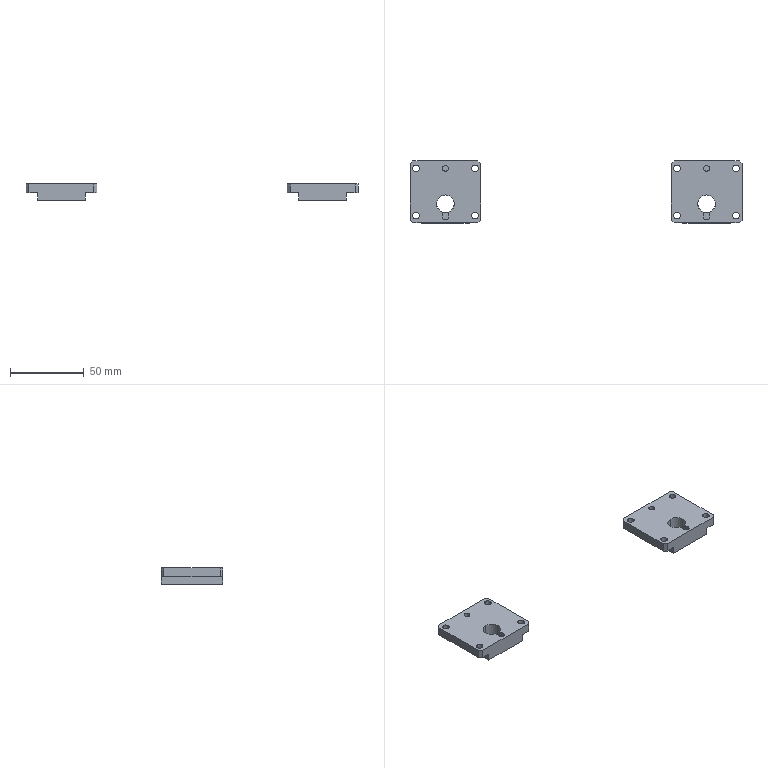Part | 2 solids | 94 faces | box 225 x 42 x 11 mm | volume 33435 mm3 | cylinder 42 | plane 36 | cone 16 | commonest cylinder face diameters 4.5 x16 4 x14 2.5 x8 12 x4